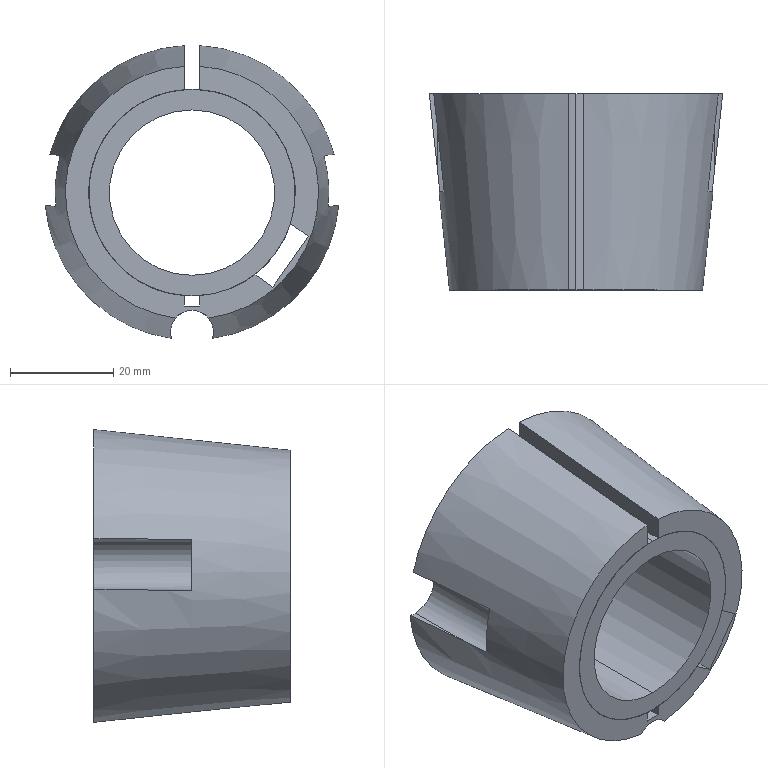Part | SolidWorks | features BaseBody 1, ICE 1 | 1 solid | 27 faces | box 56.795 x 38 x 56.678 mm | volume 48343 mm3 | plane 13 | cylinder 12 | cone 2 | commonest cylinder face diameters 10 x6 8.376 x2 32 x2 40 x2
STEP:
#1=CARTESIAN_POINT('',(0.,-0.0001031,-16.));
#2=VERTEX_POINT('',#1);
#3=CARTESIAN_POINT('',(0.,-0.0001031,16.));
#4=VERTEX_POINT('',#3);
#5=CARTESIAN_POINT('',(0.,-0.0001031,0.));
#6=DIRECTION('',(0.,1.,0.));
#7=DIRECTION('',(0.,0.,1.));
#8=AXIS2_PLACEMENT_3D('',#5,#6,#7);
#9=CIRCLE('',#8,16.);
#10=EDGE_CURVE('',#2,#4,#9,.T.);
#11=ORIENTED_EDGE('',*,*,#10,.F.);
#12=CARTESIAN_POINT('',(0.,38.,-16.));
#13=VERTEX_POINT('',#12);
#14=CARTESIAN_POINT('',(0.,-0.0001031,-16.));
#15=DIRECTION('',(0.,1.,0.));
#16=VECTOR('',#15,1000.);
#17=LINE('',#14,#16);
#18=EDGE_CURVE('',#2,#13,#17,.T.);
#19=ORIENTED_EDGE('',*,*,#18,.T.);
#20=CARTESIAN_POINT('',(0.,38.,16.));
#21=VERTEX_POINT('',#20);
#22=CARTESIAN_POINT('',(0.,38.,0.));
#23=DIRECTION('',(0.,1.,0.));
#24=DIRECTION('',(0.,0.,1.));
#25=AXIS2_PLACEMENT_3D('',#22,#23,#24);
#26=CIRCLE('',#25,16.);
#27=EDGE_CURVE('',#13,#21,#26,.T.);
#28=ORIENTED_EDGE('',*,*,#27,.T.);
#29=CARTESIAN_POINT('',(0.,-0.0001031,16.));
#30=DIRECTION('',(0.,1.,0.));
#31=VECTOR('',#30,1000.);
#32=LINE('',#29,#31);
#33=EDGE_CURVE('',#4,#21,#32,.T.);
#34=ORIENTED_EDGE('',*,*,#33,.F.);
#35=EDGE_LOOP('',(#11,#19,#28,#34));
#36=FACE_OUTER_BOUND('',#35,.T.);
#37=CARTESIAN_POINT('',(0.,-0.0001031,0.));
#38=DIRECTION('',(0.,1.,0.));
#39=DIRECTION('',(0.,0.,1.));
#40=AXIS2_PLACEMENT_3D('',#37,#38,#39);
#41=CYLINDRICAL_SURFACE('',#40,16.);
#42=ADVANCED_FACE('',(#36),#41,.F.);
#43=CARTESIAN_POINT('',(0.,-0.0001031,20.));
#44=VERTEX_POINT('',#43);
#45=CARTESIAN_POINT('',(0.,-0.0001031,-20.));
#46=VERTEX_POINT('',#45);
#47=CARTESIAN_POINT('',(0.,-0.0001031,0.));
#48=DIRECTION('',(0.,1.,0.));
#49=DIRECTION('',(0.,0.,1.));
#50=AXIS2_PLACEMENT_3D('',#47,#48,#49);
#51=CIRCLE('',#50,20.);
#52=EDGE_CURVE('',#44,#46,#51,.T.);
#53=ORIENTED_EDGE('',*,*,#52,.T.);
#54=CARTESIAN_POINT('',(0.,38.,-20.));
#55=VERTEX_POINT('',#54);
#56=CARTESIAN_POINT('',(0.,-0.0001031,-20.));
#57=DIRECTION('',(0.,1.,0.));
#58=VECTOR('',#57,1000.);
#59=LINE('',#56,#58);
#60=EDGE_CURVE('',#46,#55,#59,.T.);
#61=ORIENTED_EDGE('',*,*,#60,.T.);
#62=CARTESIAN_POINT('',(1.5,38.,-19.944));
#63=VERTEX_POINT('',#62);
#64=CARTESIAN_POINT('',(0.,38.,0.));
#65=DIRECTION('',(0.,1.,0.));
#66=DIRECTION('',(0.,0.,1.));
#67=AXIS2_PLACEMENT_3D('',#64,#65,#66);
#68=CIRCLE('',#67,20.);
#69=EDGE_CURVE('',#63,#55,#68,.T.);
#70=ORIENTED_EDGE('',*,*,#69,.F.);
#71=CARTESIAN_POINT('',(1.5,0.,-19.944));
#72=VERTEX_POINT('',#71);
#73=CARTESIAN_POINT('',(1.5,-50.,-19.944));
#74=DIRECTION('',(0.,1.,0.));
#75=VECTOR('',#74,1000.);
#76=LINE('',#73,#75);
#77=EDGE_CURVE('',#72,#63,#76,.T.);
#78=ORIENTED_EDGE('',*,*,#77,.F.);
#79=CARTESIAN_POINT('',(12.187,0.,-15.858));
#80=VERTEX_POINT('',#79);
#81=CARTESIAN_POINT('',(0.,0.,0.));
#82=DIRECTION('',(0.,1.,0.));
#83=DIRECTION('',(0.,0.,1.));
#84=AXIS2_PLACEMENT_3D('',#81,#82,#83);
#85=CIRCLE('',#84,20.);
#86=EDGE_CURVE('',#80,#72,#85,.T.);
#87=ORIENTED_EDGE('',*,*,#86,.F.);
#88=CARTESIAN_POINT('',(12.187,38.,-15.858));
#89=VERTEX_POINT('',#88);
#90=CARTESIAN_POINT('',(12.187,-462.,-15.858));
#91=DIRECTION('',(0.,1.,0.));
#92=VECTOR('',#91,1000.);
#93=LINE('',#90,#92);
#94=EDGE_CURVE('',#80,#89,#93,.T.);
#95=ORIENTED_EDGE('',*,*,#94,.T.);
#96=CARTESIAN_POINT('',(19.07,38.,-6.028));
#97=VERTEX_POINT('',#96);
#98=CARTESIAN_POINT('',(0.,38.,0.));
#99=DIRECTION('',(0.,1.,0.));
#100=DIRECTION('',(0.,0.,1.));
#101=AXIS2_PLACEMENT_3D('',#98,#99,#100);
#102=CIRCLE('',#101,20.);
#103=EDGE_CURVE('',#97,#89,#102,.T.);
#104=ORIENTED_EDGE('',*,*,#103,.F.);
#105=CARTESIAN_POINT('',(19.07,0.,-6.028));
#106=VERTEX_POINT('',#105);
#107=CARTESIAN_POINT('',(19.07,-50.,-6.028));
#108=DIRECTION('',(0.,1.,0.));
#109=VECTOR('',#108,1000.);
#110=LINE('',#107,#109);
#111=EDGE_CURVE('',#106,#97,#110,.T.);
#112=ORIENTED_EDGE('',*,*,#111,.F.);
#113=CARTESIAN_POINT('',(1.5,0.,19.944));
#114=VERTEX_POINT('',#113);
#115=CARTESIAN_POINT('',(0.,0.,0.));
#116=DIRECTION('',(0.,1.,0.));
#117=DIRECTION('',(0.,0.,1.));
#118=AXIS2_PLACEMENT_3D('',#115,#116,#117);
#119=CIRCLE('',#118,20.);
#120=EDGE_CURVE('',#114,#106,#119,.T.);
#121=ORIENTED_EDGE('',*,*,#120,.F.);
#122=CARTESIAN_POINT('',(1.5,38.,19.944));
#123=VERTEX_POINT('',#122);
#124=CARTESIAN_POINT('',(1.5,-462.,19.944));
#125=DIRECTION('',(0.,1.,0.));
#126=VECTOR('',#125,1000.);
#127=LINE('',#124,#126);
#128=EDGE_CURVE('',#114,#123,#127,.T.);
#129=ORIENTED_EDGE('',*,*,#128,.T.);
#130=CARTESIAN_POINT('',(0.,38.,20.));
#131=VERTEX_POINT('',#130);
#132=CARTESIAN_POINT('',(0.,38.,0.));
#133=DIRECTION('',(0.,1.,0.));
#134=DIRECTION('',(0.,0.,1.));
#135=AXIS2_PLACEMENT_3D('',#132,#133,#134);
#136=CIRCLE('',#135,20.);
#137=EDGE_CURVE('',#131,#123,#136,.T.);
#138=ORIENTED_EDGE('',*,*,#137,.F.);
#139=CARTESIAN_POINT('',(0.,-0.0001031,20.));
#140=DIRECTION('',(0.,1.,0.));
#141=VECTOR('',#140,1000.);
#142=LINE('',#139,#141);
#143=EDGE_CURVE('',#44,#131,#142,.T.);
#144=ORIENTED_EDGE('',*,*,#143,.F.);
#145=EDGE_LOOP('',(#53,#61,#70,#78,#87,#95,#104,#112,#121,#129,#138,#144));
#146=FACE_OUTER_BOUND('',#145,.T.);
#147=CARTESIAN_POINT('',(0.,-0.0001031,0.));
#148=DIRECTION('',(0.,1.,0.));
#149=DIRECTION('',(0.,0.,1.));
#150=AXIS2_PLACEMENT_3D('',#147,#148,#149);
#151=CYLINDRICAL_SURFACE('',#150,20.);
#152=ADVANCED_FACE('',(#146),#151,.T.);
#153=CARTESIAN_POINT('',(26.885,38.,7.352));
#154=VERTEX_POINT('',#153);
#155=CARTESIAN_POINT('',(26.885,38.,-2.648));
#156=VERTEX_POINT('',#155);
#157=CARTESIAN_POINT('',(26.885,38.,2.352));
#158=DIRECTION('',(0.,-1.,0.));
#159=DIRECTION('',(0.,0.,-1.));
#160=AXIS2_PLACEMENT_3D('',#157,#158,#159);
#161=CIRCLE('',#160,5.);
#162=EDGE_CURVE('',#154,#156,#161,.T.);
#163=ORIENTED_EDGE('',*,*,#162,.F.);
#164=CARTESIAN_POINT('',(26.885,32.025,7.352));
#165=VERTEX_POINT('',#164);
#166=CARTESIAN_POINT('',(26.885,19.,7.352));
#167=DIRECTION('',(0.,-1.,0.));
#168=VECTOR('',#167,1000.);
#169=LINE('',#166,#168);
#170=EDGE_CURVE('',#154,#165,#169,.T.);
#171=ORIENTED_EDGE('',*,*,#170,.T.);
#172=CARTESIAN_POINT('',(25.517,19.,7.161));
#173=VERTEX_POINT('',#172);
#174=CARTESIAN_POINT('',(25.517,19.,7.161));
#175=CARTESIAN_POINT('',(25.956,23.342,7.286));
#176=CARTESIAN_POINT('',(26.412,27.684,7.352));
#177=CARTESIAN_POINT('',(26.885,32.025,7.352));
#178=B_SPLINE_CURVE_WITH_KNOTS('',3,(#174,#175,#176,#177),.UNSPECIFIED.,.F.,.F.,(4,4),(0.,0.0131),.UNSPECIFIED.);
#179=EDGE_CURVE('',#173,#165,#178,.T.);
#180=ORIENTED_EDGE('',*,*,#179,.F.);
#181=CARTESIAN_POINT('',(26.373,19.,-2.622));
#182=VERTEX_POINT('',#181);
#183=CARTESIAN_POINT('',(26.885,19.,2.352));
#184=DIRECTION('',(0.,1.,0.));
#185=DIRECTION('',(0.,0.,-1.));
#186=AXIS2_PLACEMENT_3D('',#183,#184,#185);
#187=CIRCLE('',#186,5.);
#188=EDGE_CURVE('',#182,#173,#187,.T.);
#189=ORIENTED_EDGE('',*,*,#188,.F.);
#190=CARTESIAN_POINT('',(26.885,23.87,-2.648));
#191=VERTEX_POINT('',#190);
#192=CARTESIAN_POINT('',(26.885,23.87,-2.648));
#193=CARTESIAN_POINT('',(26.713,22.247,-2.648));
#194=CARTESIAN_POINT('',(26.543,20.623,-2.639));
#195=CARTESIAN_POINT('',(26.373,19.,-2.622));
#196=B_SPLINE_CURVE_WITH_KNOTS('',3,(#192,#193,#194,#195),.UNSPECIFIED.,.F.,.F.,(4,4),(0.01421,0.01911),.UNSPECIFIED.);
#197=EDGE_CURVE('',#191,#182,#196,.T.);
#198=ORIENTED_EDGE('',*,*,#197,.F.);
#199=CARTESIAN_POINT('',(26.885,19.,-2.648));
#200=DIRECTION('',(0.,-1.,0.));
#201=VECTOR('',#200,1000.);
#202=LINE('',#199,#201);
#203=EDGE_CURVE('',#156,#191,#202,.T.);
#204=ORIENTED_EDGE('',*,*,#203,.F.);
#205=EDGE_LOOP('',(#163,#171,#180,#189,#198,#204));
#206=FACE_OUTER_BOUND('',#205,.T.);
#207=CARTESIAN_POINT('',(26.885,19.,2.352));
#208=DIRECTION('',(0.,-1.,0.));
#209=DIRECTION('',(0.,0.,-1.));
#210=AXIS2_PLACEMENT_3D('',#207,#208,#209);
#211=CYLINDRICAL_SURFACE('',#210,5.);
#212=ADVANCED_FACE('',(#206),#211,.F.);
#213=CARTESIAN_POINT('',(28.398,38.,-2.414));
#214=VERTEX_POINT('',#213);
#215=CARTESIAN_POINT('',(26.885,38.,2.352));
#216=DIRECTION('',(0.,-1.,0.));
#217=DIRECTION('',(0.,0.,-1.));
#218=AXIS2_PLACEMENT_3D('',#215,#216,#217);
#219=CIRCLE('',#218,5.);
#220=EDGE_CURVE('',#156,#214,#219,.T.);
#221=ORIENTED_EDGE('',*,*,#220,.F.);
#222=ORIENTED_EDGE('',*,*,#203,.T.);
#223=CARTESIAN_POINT('',(28.398,38.,-2.414));
#224=CARTESIAN_POINT('',(27.887,33.292,-2.576));
#225=CARTESIAN_POINT('',(27.382,28.582,-2.648));
#226=CARTESIAN_POINT('',(26.885,23.87,-2.648));
#227=B_SPLINE_CURVE_WITH_KNOTS('',3,(#223,#224,#225,#226),.UNSPECIFIED.,.F.,.F.,(4,4),(0.,0.01421),.UNSPECIFIED.);
#228=EDGE_CURVE('',#214,#191,#227,.T.);
#229=ORIENTED_EDGE('',*,*,#228,.F.);
#230=EDGE_LOOP('',(#221,#222,#229));
#231=FACE_OUTER_BOUND('',#230,.T.);
#232=CARTESIAN_POINT('',(26.885,19.,2.352));
#233=DIRECTION('',(0.,-1.,0.));
#234=DIRECTION('',(0.,0.,-1.));
#235=AXIS2_PLACEMENT_3D('',#232,#233,#234);
#236=CYLINDRICAL_SURFACE('',#235,5.);
#237=ADVANCED_FACE('',(#231),#236,.F.);
#238=CARTESIAN_POINT('',(0.,0.,-22.8));
#239=VERTEX_POINT('',#238);
#240=CARTESIAN_POINT('',(3.208,0.,-24.295));
#241=VERTEX_POINT('',#240);
#242=CARTESIAN_POINT('',(0.,0.,-26.988));
#243=DIRECTION('',(0.,1.,0.));
#244=DIRECTION('',(0.,0.,1.));
#245=AXIS2_PLACEMENT_3D('',#242,#243,#244);
#246=CIRCLE('',#245,4.188);
#247=EDGE_CURVE('',#239,#241,#246,.T.);
#248=ORIENTED_EDGE('',*,*,#247,.F.);
#249=CARTESIAN_POINT('',(0.,38.,-22.8));
#250=VERTEX_POINT('',#249);
#251=CARTESIAN_POINT('',(0.,0.,-22.8));
#252=DIRECTION('',(0.,1.,0.));
#253=VECTOR('',#252,1000.);
#254=LINE('',#251,#253);
#255=EDGE_CURVE('',#239,#250,#254,.T.);
#256=ORIENTED_EDGE('',*,*,#255,.T.);
#257=CARTESIAN_POINT('',(4.003,38.,-28.217));
#258=VERTEX_POINT('',#257);
#259=CARTESIAN_POINT('',(0.,38.,-26.988));
#260=DIRECTION('',(0.,-1.,0.));
#261=DIRECTION('',(0.,0.,1.));
#262=AXIS2_PLACEMENT_3D('',#259,#260,#261);
#263=CIRCLE('',#262,4.188);
#264=EDGE_CURVE('',#258,#250,#263,.T.);
#265=ORIENTED_EDGE('',*,*,#264,.F.);
#266=CARTESIAN_POINT('',(3.208,0.,-24.295));
#267=CARTESIAN_POINT('',(3.461,3.163,-24.597));
#268=CARTESIAN_POINT('',(3.65,6.33,-24.905));
#269=CARTESIAN_POINT('',(3.943,12.665,-25.535));
#270=CARTESIAN_POINT('',(4.046,15.833,-25.855));
#271=CARTESIAN_POINT('',(4.174,22.167,-26.509));
#272=CARTESIAN_POINT('',(4.199,25.334,-26.842));
#273=CARTESIAN_POINT('',(4.168,31.667,-27.521));
#274=CARTESIAN_POINT('',(4.111,34.834,-27.866));
#275=CARTESIAN_POINT('',(4.003,38.,-28.217));
#276=B_SPLINE_CURVE_WITH_KNOTS('',3,(#266,#267,#268,#269,#270,#271,#272,#273,#274,#275),.UNSPECIFIED.,.F.,.F.,(4,2,2,2,4),(0.,0.009561,0.01912,0.02868,0.03824),.UNSPECIFIED.);
#277=EDGE_CURVE('',#241,#258,#276,.T.);
#278=ORIENTED_EDGE('',*,*,#277,.F.);
#279=EDGE_LOOP('',(#248,#256,#265,#278));
#280=FACE_OUTER_BOUND('',#279,.T.);
#281=CARTESIAN_POINT('',(0.,0.,-26.988));
#282=DIRECTION('',(0.,1.,0.));
#283=DIRECTION('',(0.,0.,1.));
#284=AXIS2_PLACEMENT_3D('',#281,#282,#283);
#285=CYLINDRICAL_SURFACE('',#284,4.188);
#286=ADVANCED_FACE('',(#280),#285,.F.);
#287=CARTESIAN_POINT('',(-26.885,38.,7.352));
#288=VERTEX_POINT('',#287);
#289=CARTESIAN_POINT('',(-27.547,38.,7.308));
#290=VERTEX_POINT('',#289);
#291=CARTESIAN_POINT('',(-26.885,38.,2.352));
#292=DIRECTION('',(0.,-1.,0.));
#293=DIRECTION('',(0.,0.,-1.));
#294=AXIS2_PLACEMENT_3D('',#291,#292,#293);
#295=CIRCLE('',#294,5.);
#296=EDGE_CURVE('',#288,#290,#295,.T.);
#297=ORIENTED_EDGE('',*,*,#296,.F.);
#298=CARTESIAN_POINT('',(-26.885,32.025,7.352));
#299=VERTEX_POINT('',#298);
#300=CARTESIAN_POINT('',(-26.885,19.,7.352));
#301=DIRECTION('',(0.,-1.,0.));
#302=VECTOR('',#301,1000.);
#303=LINE('',#300,#302);
#304=EDGE_CURVE('',#288,#299,#303,.T.);
#305=ORIENTED_EDGE('',*,*,#304,.T.);
#306=CARTESIAN_POINT('',(-27.547,38.,7.308));
#307=CARTESIAN_POINT('',(-27.323,36.009,7.338));
#308=CARTESIAN_POINT('',(-27.102,34.017,7.352));
#309=CARTESIAN_POINT('',(-26.885,32.025,7.352));
#310=B_SPLINE_CURVE_WITH_KNOTS('',3,(#306,#307,#308,#309),.UNSPECIFIED.,.F.,.F.,(4,4),(0.,0.006012),.UNSPECIFIED.);
#311=EDGE_CURVE('',#290,#299,#310,.T.);
#312=ORIENTED_EDGE('',*,*,#311,.F.);
#313=EDGE_LOOP('',(#297,#305,#312));
#314=FACE_OUTER_BOUND('',#313,.T.);
#315=CARTESIAN_POINT('',(-26.885,19.,2.352));
#316=DIRECTION('',(0.,-1.,0.));
#317=DIRECTION('',(0.,0.,-1.));
#318=AXIS2_PLACEMENT_3D('',#315,#316,#317);
#319=CYLINDRICAL_SURFACE('',#318,5.);
#320=ADVANCED_FACE('',(#314),#319,.F.);
#321=ORIENTED_EDGE('',*,*,#304,.F.);
#322=CARTESIAN_POINT('',(-26.885,38.,-2.648));
#323=VERTEX_POINT('',#322);
#324=CARTESIAN_POINT('',(-26.885,38.,2.352));
#325=DIRECTION('',(0.,-1.,0.));
#326=DIRECTION('',(0.,0.,-1.));
#327=AXIS2_PLACEMENT_3D('',#324,#325,#326);
#328=CIRCLE('',#327,5.);
#329=EDGE_CURVE('',#323,#288,#328,.T.);
#330=ORIENTED_EDGE('',*,*,#329,.F.);
#331=CARTESIAN_POINT('',(-26.885,23.87,-2.648));
#332=VERTEX_POINT('',#331);
#333=CARTESIAN_POINT('',(-26.885,19.,-2.648));
#334=DIRECTION('',(0.,-1.,0.));
#335=VECTOR('',#334,1000.);
#336=LINE('',#333,#335);
#337=EDGE_CURVE('',#323,#332,#336,.T.);
#338=ORIENTED_EDGE('',*,*,#337,.T.);
#339=CARTESIAN_POINT('',(-26.373,19.,-2.622));
#340=VERTEX_POINT('',#339);
#341=CARTESIAN_POINT('',(-26.373,19.,-2.622));
#342=CARTESIAN_POINT('',(-26.543,20.623,-2.639));
#343=CARTESIAN_POINT('',(-26.713,22.247,-2.648));
#344=CARTESIAN_POINT('',(-26.885,23.87,-2.648));
#345=B_SPLINE_CURVE_WITH_KNOTS('',3,(#341,#342,#343,#344),.UNSPECIFIED.,.F.,.F.,(4,4),(0.,0.004897),.UNSPECIFIED.);
#346=EDGE_CURVE('',#340,#332,#345,.T.);
#347=ORIENTED_EDGE('',*,*,#346,.F.);
#348=CARTESIAN_POINT('',(-25.517,19.,7.161));
#349=VERTEX_POINT('',#348);
#350=CARTESIAN_POINT('',(-26.885,19.,2.352));
#351=DIRECTION('',(0.,1.,0.));
#352=DIRECTION('',(0.,0.,-1.));
#353=AXIS2_PLACEMENT_3D('',#350,#351,#352);
#354=CIRCLE('',#353,5.);
#355=EDGE_CURVE('',#349,#340,#354,.T.);
#356=ORIENTED_EDGE('',*,*,#355,.F.);
#357=CARTESIAN_POINT('',(-26.885,32.025,7.352));
#358=CARTESIAN_POINT('',(-26.412,27.684,7.352));
#359=CARTESIAN_POINT('',(-25.956,23.342,7.286));
#360=CARTESIAN_POINT('',(-25.517,19.,7.161));
#361=B_SPLINE_CURVE_WITH_KNOTS('',3,(#357,#358,#359,#360),.UNSPECIFIED.,.F.,.F.,(4,4),(0.006012,0.01911),.UNSPECIFIED.);
#362=EDGE_CURVE('',#299,#349,#361,.T.);
#363=ORIENTED_EDGE('',*,*,#362,.F.);
#364=EDGE_LOOP('',(#321,#330,#338,#347,#356,#363));
#365=FACE_OUTER_BOUND('',#364,.T.);
#366=CARTESIAN_POINT('',(-26.885,19.,2.352));
#367=DIRECTION('',(0.,-1.,0.));
#368=DIRECTION('',(0.,0.,-1.));
#369=AXIS2_PLACEMENT_3D('',#366,#367,#368);
#370=CYLINDRICAL_SURFACE('',#369,5.);
#371=ADVANCED_FACE('',(#365),#370,.F.);
#372=ORIENTED_EDGE('',*,*,#228,.T.);
#373=ORIENTED_EDGE('',*,*,#197,.T.);
#374=CARTESIAN_POINT('',(0.,19.,0.));
#375=DIRECTION('',(0.,-1.,0.));
#376=DIRECTION('',(0.,0.,1.));
#377=AXIS2_PLACEMENT_3D('',#374,#375,#376);
#378=CIRCLE('',#377,26.503);
#379=EDGE_CURVE('',#182,#173,#378,.T.);
#380=ORIENTED_EDGE('',*,*,#379,.T.);
#381=ORIENTED_EDGE('',*,*,#179,.T.);
#382=CARTESIAN_POINT('',(27.547,38.,7.308));
#383=VERTEX_POINT('',#382);
#384=CARTESIAN_POINT('',(26.885,32.025,7.352));
#385=CARTESIAN_POINT('',(27.102,34.017,7.352));
#386=CARTESIAN_POINT('',(27.323,36.009,7.338));
#387=CARTESIAN_POINT('',(27.547,38.,7.308));
#388=B_SPLINE_CURVE_WITH_KNOTS('',3,(#384,#385,#386,#387),.UNSPECIFIED.,.F.,.F.,(4,4),(0.0131,0.01911),.UNSPECIFIED.);
#389=EDGE_CURVE('',#165,#383,#388,.T.);
#390=ORIENTED_EDGE('',*,*,#389,.T.);
#391=CARTESIAN_POINT('',(1.5,38.,28.46));
#392=VERTEX_POINT('',#391);
#393=CARTESIAN_POINT('',(0.,38.,0.));
#394=DIRECTION('',(0.,-1.,0.));
#395=DIRECTION('',(0.,0.,1.));
#396=AXIS2_PLACEMENT_3D('',#393,#394,#395);
#397=CIRCLE('',#396,28.5);
#398=EDGE_CURVE('',#383,#392,#397,.T.);
#399=ORIENTED_EDGE('',*,*,#398,.T.);
#400=CARTESIAN_POINT('',(1.5,0.,24.46));
#401=VERTEX_POINT('',#400);
#402=CARTESIAN_POINT('',(1.5,38.,28.46));
#403=CARTESIAN_POINT('',(1.5,25.333,27.127));
#404=CARTESIAN_POINT('',(1.5,12.667,25.794));
#405=CARTESIAN_POINT('',(1.5,0.,24.46));
#406=B_SPLINE_CURVE_WITH_KNOTS('',3,(#402,#403,#404,#405),.UNSPECIFIED.,.F.,.F.,(4,4),(0.,0.03821),.UNSPECIFIED.);
#407=EDGE_CURVE('',#392,#401,#406,.T.);
#408=ORIENTED_EDGE('',*,*,#407,.T.);
#409=CARTESIAN_POINT('',(0.,0.,0.));
#410=DIRECTION('',(0.,1.,0.));
#411=DIRECTION('',(0.,0.,1.));
#412=AXIS2_PLACEMENT_3D('',#409,#410,#411);
#413=CIRCLE('',#412,24.506);
#414=EDGE_CURVE('',#401,#241,#413,.T.);
#415=ORIENTED_EDGE('',*,*,#414,.T.);
#416=ORIENTED_EDGE('',*,*,#277,.T.);
#417=CARTESIAN_POINT('',(0.,38.,0.));
#418=DIRECTION('',(0.,-1.,0.));
#419=DIRECTION('',(0.,0.,1.));
#420=AXIS2_PLACEMENT_3D('',#417,#418,#419);
#421=CIRCLE('',#420,28.5);
#422=EDGE_CURVE('',#258,#214,#421,.T.);
#423=ORIENTED_EDGE('',*,*,#422,.T.);
#424=EDGE_LOOP('',(#372,#373,#380,#381,#390,#399,#408,#415,#416,#423));
#425=FACE_OUTER_BOUND('',#424,.T.);
#426=CARTESIAN_POINT('',(0.,38.,0.));
#427=DIRECTION('',(0.,1.,0.));
#428=DIRECTION('',(0.,0.,1.));
#429=AXIS2_PLACEMENT_3D('',#426,#427,#428);
#430=CONICAL_SURFACE('',#429,28.5,0.1047);
#431=ADVANCED_FACE('',(#425),#430,.T.);
#432=ORIENTED_EDGE('',*,*,#188,.T.);
#433=ORIENTED_EDGE('',*,*,#379,.F.);
#434=EDGE_LOOP('',(#432,#433));
#435=FACE_OUTER_BOUND('',#434,.T.);
#436=CARTESIAN_POINT('',(0.,19.,0.));
#437=DIRECTION('',(0.,1.,0.));
#438=DIRECTION('',(0.,0.,1.));
#439=AXIS2_PLACEMENT_3D('',#436,#437,#438);
#440=PLANE('',#439);
#441=ADVANCED_FACE('',(#435),#440,.T.);
#442=ORIENTED_EDGE('',*,*,#170,.F.);
#443=CARTESIAN_POINT('',(26.885,38.,2.352));
#444=DIRECTION('',(0.,-1.,0.));
#445=DIRECTION('',(0.,0.,-1.));
#446=AXIS2_PLACEMENT_3D('',#443,#444,#445);
#447=CIRCLE('',#446,5.);
#448=EDGE_CURVE('',#383,#154,#447,.T.);
#449=ORIENTED_EDGE('',*,*,#448,.F.);
#450=ORIENTED_EDGE('',*,*,#389,.F.);
#451=EDGE_LOOP('',(#442,#449,#450));
#452=FACE_OUTER_BOUND('',#451,.T.);
#453=CARTESIAN_POINT('',(26.885,19.,2.352));
#454=DIRECTION('',(0.,-1.,0.));
#455=DIRECTION('',(0.,0.,-1.));
#456=AXIS2_PLACEMENT_3D('',#453,#454,#455);
#457=CYLINDRICAL_SURFACE('',#456,5.);
#458=ADVANCED_FACE('',(#452),#457,.F.);
#459=CARTESIAN_POINT('',(-1.5,38.,19.944));
#460=VERTEX_POINT('',#459);
#461=CARTESIAN_POINT('',(0.,38.,0.));
#462=DIRECTION('',(0.,1.,0.));
#463=DIRECTION('',(0.,0.,1.));
#464=AXIS2_PLACEMENT_3D('',#461,#462,#463);
#465=CIRCLE('',#464,20.);
#466=EDGE_CURVE('',#460,#131,#465,.T.);
#467=ORIENTED_EDGE('',*,*,#466,.T.);
#468=ORIENTED_EDGE('',*,*,#137,.T.);
#469=CARTESIAN_POINT('',(1.5,38.,0.));
#470=DIRECTION('',(0.,0.,1.));
#471=VECTOR('',#470,1000.);
#472=LINE('',#469,#471);
#473=EDGE_CURVE('',#123,#392,#472,.T.);
#474=ORIENTED_EDGE('',*,*,#473,.T.);
#475=ORIENTED_EDGE('',*,*,#398,.F.);
#476=ORIENTED_EDGE('',*,*,#448,.T.);
#477=ORIENTED_EDGE('',*,*,#162,.T.);
#478=ORIENTED_EDGE('',*,*,#220,.T.);
#479=ORIENTED_EDGE('',*,*,#422,.F.);
#480=ORIENTED_EDGE('',*,*,#264,.T.);
#481=CARTESIAN_POINT('',(-4.003,38.,-28.217));
#482=VERTEX_POINT('',#481);
#483=CARTESIAN_POINT('',(0.,38.,-26.988));
#484=DIRECTION('',(0.,-1.,0.));
#485=DIRECTION('',(0.,0.,1.));
#486=AXIS2_PLACEMENT_3D('',#483,#484,#485);
#487=CIRCLE('',#486,4.188);
#488=EDGE_CURVE('',#250,#482,#487,.T.);
#489=ORIENTED_EDGE('',*,*,#488,.T.);
#490=CARTESIAN_POINT('',(-28.398,38.,-2.414));
#491=VERTEX_POINT('',#490);
#492=CARTESIAN_POINT('',(0.,38.,0.));
#493=DIRECTION('',(0.,1.,0.));
#494=DIRECTION('',(0.,0.,1.));
#495=AXIS2_PLACEMENT_3D('',#492,#493,#494);
#496=CIRCLE('',#495,28.5);
#497=EDGE_CURVE('',#482,#491,#496,.T.);
#498=ORIENTED_EDGE('',*,*,#497,.T.);
#499=CARTESIAN_POINT('',(-26.885,38.,2.352));
#500=DIRECTION('',(0.,-1.,0.));
#501=DIRECTION('',(0.,0.,-1.));
#502=AXIS2_PLACEMENT_3D('',#499,#500,#501);
#503=CIRCLE('',#502,5.);
#504=EDGE_CURVE('',#491,#323,#503,.T.);
#505=ORIENTED_EDGE('',*,*,#504,.T.);
#506=ORIENTED_EDGE('',*,*,#329,.T.);
#507=ORIENTED_EDGE('',*,*,#296,.T.);
#508=CARTESIAN_POINT('',(-1.5,38.,28.46));
#509=VERTEX_POINT('',#508);
#510=CARTESIAN_POINT('',(0.,38.,0.));
#511=DIRECTION('',(0.,1.,0.));
#512=DIRECTION('',(0.,0.,1.));
#513=AXIS2_PLACEMENT_3D('',#510,#511,#512);
#514=CIRCLE('',#513,28.5);
#515=EDGE_CURVE('',#290,#509,#514,.T.);
#516=ORIENTED_EDGE('',*,*,#515,.T.);
#517=CARTESIAN_POINT('',(-1.5,38.,0.));
#518=DIRECTION('',(0.,0.,-1.));
#519=VECTOR('',#518,1000.);
#520=LINE('',#517,#519);
#521=EDGE_CURVE('',#509,#460,#520,.T.);
#522=ORIENTED_EDGE('',*,*,#521,.T.);
#523=EDGE_LOOP('',(#467,#468,#474,#475,#476,#477,#478,#479,#480,#489,#498,#505,#506,#507,#516,#522));
#524=FACE_OUTER_BOUND('',#523,.T.);
#525=ORIENTED_EDGE('',*,*,#103,.T.);
#526=CARTESIAN_POINT('',(15.645,38.,-18.279));
#527=VERTEX_POINT('',#526);
#528=CARTESIAN_POINT('',(12.187,38.,-15.858));
#529=DIRECTION('',(0.8192,0.,-0.5736));
#530=VECTOR('',#529,1000.);
#531=LINE('',#528,#530);
#532=EDGE_CURVE('',#89,#527,#531,.T.);
#533=ORIENTED_EDGE('',*,*,#532,.T.);
#534=CARTESIAN_POINT('',(22.528,38.,-8.449));
#535=VERTEX_POINT('',#534);
#536=CARTESIAN_POINT('',(15.645,38.,-18.279));
#537=DIRECTION('',(0.5736,0.,0.8192));
#538=VECTOR('',#537,1000.);
#539=LINE('',#536,#538);
#540=EDGE_CURVE('',#527,#535,#539,.T.);
#541=ORIENTED_EDGE('',*,*,#540,.T.);
#542=CARTESIAN_POINT('',(22.528,38.,-8.449));
#543=DIRECTION('',(-0.8192,0.,0.5736));
#544=VECTOR('',#543,1000.);
#545=LINE('',#542,#544);
#546=EDGE_CURVE('',#535,#97,#545,.T.);
#547=ORIENTED_EDGE('',*,*,#546,.T.);
#548=EDGE_LOOP('',(#525,#533,#541,#547));
#549=FACE_BOUND('',#548,.T.);
#550=CARTESIAN_POINT('',(1.5,38.,-21.949));
#551=VERTEX_POINT('',#550);
#552=CARTESIAN_POINT('',(1.5,38.,0.));
#553=DIRECTION('',(0.,0.,1.));
#554=VECTOR('',#553,1000.);
#555=LINE('',#552,#554);
#556=EDGE_CURVE('',#551,#63,#555,.T.);
#557=ORIENTED_EDGE('',*,*,#556,.T.);
#558=ORIENTED_EDGE('',*,*,#69,.T.);
#559=CARTESIAN_POINT('',(-1.5,38.,-19.944));
#560=VERTEX_POINT('',#559);
#561=CARTESIAN_POINT('',(0.,38.,0.));
#562=DIRECTION('',(0.,1.,0.));
#563=DIRECTION('',(0.,0.,1.));
#564=AXIS2_PLACEMENT_3D('',#561,#562,#563);
#565=CIRCLE('',#564,20.);
#566=EDGE_CURVE('',#55,#560,#565,.T.);
#567=ORIENTED_EDGE('',*,*,#566,.T.);
#568=CARTESIAN_POINT('',(-1.5,38.,-21.949));
#569=VERTEX_POINT('',#568);
#570=CARTESIAN_POINT('',(-1.5,38.,0.));
#571=DIRECTION('',(0.,0.,-1.));
#572=VECTOR('',#571,1000.);
#573=LINE('',#570,#572);
#574=EDGE_CURVE('',#560,#569,#573,.T.);
#575=ORIENTED_EDGE('',*,*,#574,.T.);
#576=CARTESIAN_POINT('',(28.5,38.,-21.949));
#577=DIRECTION('',(1.,0.,0.));
#578=VECTOR('',#577,1000.);
#579=LINE('',#576,#578);
#580=EDGE_CURVE('',#569,#551,#579,.T.);
#581=ORIENTED_EDGE('',*,*,#580,.T.);
#582=EDGE_LOOP('',(#557,#558,#567,#575,#581));
#583=FACE_BOUND('',#582,.T.);
#584=CARTESIAN_POINT('',(0.,38.,0.));
#585=DIRECTION('',(0.,1.,0.));
#586=DIRECTION('',(0.,0.,1.));
#587=AXIS2_PLACEMENT_3D('',#584,#585,#586);
#588=CIRCLE('',#587,16.);
#589=EDGE_CURVE('',#21,#13,#588,.T.);
#590=ORIENTED_EDGE('',*,*,#589,.F.);
#591=ORIENTED_EDGE('',*,*,#27,.F.);
#592=EDGE_LOOP('',(#590,#591));
#593=FACE_BOUND('',#592,.T.);
#594=CARTESIAN_POINT('',(28.5,38.,0.));
#595=DIRECTION('',(0.,1.,0.));
#596=DIRECTION('',(0.,0.,1.));
#597=AXIS2_PLACEMENT_3D('',#594,#595,#596);
#598=PLANE('',#597);
#599=ADVANCED_FACE('',(#524,#549,#583,#593),#598,.T.);
#600=ORIENTED_EDGE('',*,*,#255,.F.);
#601=CARTESIAN_POINT('',(-3.208,0.,-24.295));
#602=VERTEX_POINT('',#601);
#603=CARTESIAN_POINT('',(0.,0.,-26.988));
#604=DIRECTION('',(0.,1.,0.));
#605=DIRECTION('',(0.,0.,1.));
#606=AXIS2_PLACEMENT_3D('',#603,#604,#605);
#607=CIRCLE('',#606,4.188);
#608=EDGE_CURVE('',#602,#239,#607,.T.);
#609=ORIENTED_EDGE('',*,*,#608,.F.);
#610=CARTESIAN_POINT('',(-4.003,38.,-28.217));
#611=CARTESIAN_POINT('',(-4.111,34.834,-27.866));
#612=CARTESIAN_POINT('',(-4.168,31.666,-27.521));
#613=CARTESIAN_POINT('',(-4.199,25.329,-26.842));
#614=CARTESIAN_POINT('',(-4.174,22.161,-26.509));
#615=CARTESIAN_POINT('',(-4.046,15.827,-25.855));
#616=CARTESIAN_POINT('',(-3.943,12.66,-25.534));
#617=CARTESIAN_POINT('',(-3.65,6.329,-24.905));
#618=CARTESIAN_POINT('',(-3.461,3.164,-24.597));
#619=CARTESIAN_POINT('',(-3.208,0.,-24.295));
#620=B_SPLINE_CURVE_WITH_KNOTS('',3,(#610,#611,#612,#613,#614,#615,#616,#617,#618,#619),.UNSPECIFIED.,.F.,.F.,(4,2,2,2,4),(0.,0.009561,0.01912,0.02868,0.03824),.UNSPECIFIED.);
#621=EDGE_CURVE('',#482,#602,#620,.T.);
#622=ORIENTED_EDGE('',*,*,#621,.F.);
#623=ORIENTED_EDGE('',*,*,#488,.F.);
#624=EDGE_LOOP('',(#600,#609,#622,#623));
#625=FACE_OUTER_BOUND('',#624,.T.);
#626=CARTESIAN_POINT('',(0.,0.,-26.988));
#627=DIRECTION('',(0.,1.,0.));
#628=DIRECTION('',(0.,0.,1.));
#629=AXIS2_PLACEMENT_3D('',#626,#627,#628);
#630=CYLINDRICAL_SURFACE('',#629,4.188);
#631=ADVANCED_FACE('',(#625),#630,.F.);
#632=ORIENTED_EDGE('',*,*,#608,.T.);
#633=ORIENTED_EDGE('',*,*,#247,.T.);
#634=ORIENTED_EDGE('',*,*,#414,.F.);
#635=CARTESIAN_POINT('',(1.5,0.,0.));
#636=DIRECTION('',(0.,0.,-1.));
#637=VECTOR('',#636,1000.);
#638=LINE('',#635,#637);
#639=EDGE_CURVE('',#401,#114,#638,.T.);
#640=ORIENTED_EDGE('',*,*,#639,.T.);
#641=ORIENTED_EDGE('',*,*,#120,.T.);
#642=CARTESIAN_POINT('',(22.528,0.,-8.449));
#643=VERTEX_POINT('',#642);
#644=CARTESIAN_POINT('',(19.07,0.,-6.028));
#645=DIRECTION('',(0.8192,0.,-0.5736));
#646=VECTOR('',#645,1000.);
#647=LINE('',#644,#646);
#648=EDGE_CURVE('',#106,#643,#647,.T.);
#649=ORIENTED_EDGE('',*,*,#648,.T.);
#650=CARTESIAN_POINT('',(15.645,0.,-18.279));
#651=VERTEX_POINT('',#650);
#652=CARTESIAN_POINT('',(22.528,0.,-8.449));
#653=DIRECTION('',(-0.5736,0.,-0.8192));
#654=VECTOR('',#653,1000.);
#655=LINE('',#652,#654);
#656=EDGE_CURVE('',#643,#651,#655,.T.);
#657=ORIENTED_EDGE('',*,*,#656,.T.);
#658=CARTESIAN_POINT('',(15.645,0.,-18.279));
#659=DIRECTION('',(-0.8192,0.,0.5736));
#660=VECTOR('',#659,1000.);
#661=LINE('',#658,#660);
#662=EDGE_CURVE('',#651,#80,#661,.T.);
#663=ORIENTED_EDGE('',*,*,#662,.T.);
#664=ORIENTED_EDGE('',*,*,#86,.T.);
#665=CARTESIAN_POINT('',(1.5,0.,-21.949));
#666=VERTEX_POINT('',#665);
#667=CARTESIAN_POINT('',(1.5,0.,0.));
#668=DIRECTION('',(0.,0.,-1.));
#669=VECTOR('',#668,1000.);
#670=LINE('',#667,#669);
#671=EDGE_CURVE('',#72,#666,#670,.T.);
#672=ORIENTED_EDGE('',*,*,#671,.T.);
#673=CARTESIAN_POINT('',(-1.5,0.,-21.949));
#674=VERTEX_POINT('',#673);
#675=CARTESIAN_POINT('',(20.,0.,-21.949));
#676=DIRECTION('',(-1.,0.,0.));
#677=VECTOR('',#676,1000.);
#678=LINE('',#675,#677);
#679=EDGE_CURVE('',#666,#674,#678,.T.);
#680=ORIENTED_EDGE('',*,*,#679,.T.);
#681=CARTESIAN_POINT('',(-1.5,0.,-19.944));
#682=VERTEX_POINT('',#681);
#683=CARTESIAN_POINT('',(-1.5,0.,0.));
#684=DIRECTION('',(0.,0.,1.));
#685=VECTOR('',#684,1000.);
#686=LINE('',#683,#685);
#687=EDGE_CURVE('',#674,#682,#686,.T.);
#688=ORIENTED_EDGE('',*,*,#687,.T.);
#689=CARTESIAN_POINT('',(-1.5,0.,19.944));
#690=VERTEX_POINT('',#689);
#691=CARTESIAN_POINT('',(0.,0.,0.));
#692=DIRECTION('',(0.,1.,0.));
#693=DIRECTION('',(0.,0.,1.));
#694=AXIS2_PLACEMENT_3D('',#691,#692,#693);
#695=CIRCLE('',#694,20.);
#696=EDGE_CURVE('',#682,#690,#695,.T.);
#697=ORIENTED_EDGE('',*,*,#696,.T.);
#698=CARTESIAN_POINT('',(-1.5,0.,24.46));
#699=VERTEX_POINT('',#698);
#700=CARTESIAN_POINT('',(-1.5,0.,0.));
#701=DIRECTION('',(0.,0.,1.));
#702=VECTOR('',#701,1000.);
#703=LINE('',#700,#702);
#704=EDGE_CURVE('',#690,#699,#703,.T.);
#705=ORIENTED_EDGE('',*,*,#704,.T.);
#706=CARTESIAN_POINT('',(0.,0.,0.));
#707=DIRECTION('',(0.,-1.,0.));
#708=DIRECTION('',(0.,0.,1.));
#709=AXIS2_PLACEMENT_3D('',#706,#707,#708);
#710=CIRCLE('',#709,24.506);
#711=EDGE_CURVE('',#699,#602,#710,.T.);
#712=ORIENTED_EDGE('',*,*,#711,.T.);
#713=EDGE_LOOP('',(#632,#633,#634,#640,#641,#649,#657,#663,#664,#672,#680,#688,#697,#705,#712));
#714=FACE_OUTER_BOUND('',#713,.T.);
#715=CARTESIAN_POINT('',(20.,0.,0.));
#716=DIRECTION('',(0.,-1.,0.));
#717=DIRECTION('',(0.,0.,-1.));
#718=AXIS2_PLACEMENT_3D('',#715,#716,#717);
#719=PLANE('',#718);
#720=ADVANCED_FACE('',(#714),#719,.T.);
#721=ORIENTED_EDGE('',*,*,#407,.F.);
#722=ORIENTED_EDGE('',*,*,#473,.F.);
#723=ORIENTED_EDGE('',*,*,#128,.F.);
#724=ORIENTED_EDGE('',*,*,#639,.F.);
#725=EDGE_LOOP('',(#721,#722,#723,#724));
#726=FACE_OUTER_BOUND('',#725,.T.);
#727=CARTESIAN_POINT('',(1.5,-462.,28.46));
#728=DIRECTION('',(1.,0.,0.));
#729=DIRECTION('',(0.,0.,-1.));
#730=AXIS2_PLACEMENT_3D('',#727,#728,#729);
#731=PLANE('',#730);
#732=ADVANCED_FACE('',(#726),#731,.F.);
#733=ORIENTED_EDGE('',*,*,#111,.T.);
#734=ORIENTED_EDGE('',*,*,#546,.F.);
#735=CARTESIAN_POINT('',(22.528,-462.,-8.449));
#736=DIRECTION('',(0.,1.,0.));
#737=VECTOR('',#736,1000.);
#738=LINE('',#735,#737);
#739=EDGE_CURVE('',#643,#535,#738,.T.);
#740=ORIENTED_EDGE('',*,*,#739,.F.);
#741=ORIENTED_EDGE('',*,*,#648,.F.);
#742=EDGE_LOOP('',(#733,#734,#740,#741));
#743=FACE_OUTER_BOUND('',#742,.T.);
#744=CARTESIAN_POINT('',(19.07,-462.,-6.028));
#745=DIRECTION('',(0.5736,0.,0.8192));
#746=DIRECTION('',(0.8192,0.,-0.5736));
#747=AXIS2_PLACEMENT_3D('',#744,#745,#746);
#748=PLANE('',#747);
#749=ADVANCED_FACE('',(#743),#748,.F.);
#750=ORIENTED_EDGE('',*,*,#739,.T.);
#751=ORIENTED_EDGE('',*,*,#540,.F.);
#752=CARTESIAN_POINT('',(15.645,-462.,-18.279));
#753=DIRECTION('',(0.,1.,0.));
#754=VECTOR('',#753,1000.);
#755=LINE('',#752,#754);
#756=EDGE_CURVE('',#651,#527,#755,.T.);
#757=ORIENTED_EDGE('',*,*,#756,.F.);
#758=ORIENTED_EDGE('',*,*,#656,.F.);
#759=EDGE_LOOP('',(#750,#751,#757,#758));
#760=FACE_OUTER_BOUND('',#759,.T.);
#761=CARTESIAN_POINT('',(22.528,-462.,-8.449));
#762=DIRECTION('',(0.8192,0.,-0.5736));
#763=DIRECTION('',(-0.5736,0.,-0.8192));
#764=AXIS2_PLACEMENT_3D('',#761,#762,#763);
#765=PLANE('',#764);
#766=ADVANCED_FACE('',(#760),#765,.F.);
#767=ORIENTED_EDGE('',*,*,#756,.T.);
#768=ORIENTED_EDGE('',*,*,#532,.F.);
#769=ORIENTED_EDGE('',*,*,#94,.F.);
#770=ORIENTED_EDGE('',*,*,#662,.F.);
#771=EDGE_LOOP('',(#767,#768,#769,#770));
#772=FACE_OUTER_BOUND('',#771,.T.);
#773=CARTESIAN_POINT('',(15.645,-462.,-18.279));
#774=DIRECTION('',(-0.5736,0.,-0.8192));
#775=DIRECTION('',(-0.8192,0.,0.5736));
#776=AXIS2_PLACEMENT_3D('',#773,#774,#775);
#777=PLANE('',#776);
#778=ADVANCED_FACE('',(#772),#777,.F.);
#779=ORIENTED_EDGE('',*,*,#77,.T.);
#780=ORIENTED_EDGE('',*,*,#556,.F.);
#781=CARTESIAN_POINT('',(1.5,-462.,-21.949));
#782=DIRECTION('',(0.,1.,0.));
#783=VECTOR('',#782,1000.);
#784=LINE('',#781,#783);
#785=EDGE_CURVE('',#666,#551,#784,.T.);
#786=ORIENTED_EDGE('',*,*,#785,.F.);
#787=ORIENTED_EDGE('',*,*,#671,.F.);
#788=EDGE_LOOP('',(#779,#780,#786,#787));
#789=FACE_OUTER_BOUND('',#788,.T.);
#790=CARTESIAN_POINT('',(1.5,-462.,-19.944));
#791=DIRECTION('',(1.,0.,0.));
#792=DIRECTION('',(0.,0.,-1.));
#793=AXIS2_PLACEMENT_3D('',#790,#791,#792);
#794=PLANE('',#793);
#795=ADVANCED_FACE('',(#789),#794,.F.);
#796=ORIENTED_EDGE('',*,*,#785,.T.);
#797=ORIENTED_EDGE('',*,*,#580,.F.);
#798=CARTESIAN_POINT('',(-1.5,-462.,-21.949));
#799=DIRECTION('',(0.,1.,0.));
#800=VECTOR('',#799,1000.);
#801=LINE('',#798,#800);
#802=EDGE_CURVE('',#674,#569,#801,.T.);
#803=ORIENTED_EDGE('',*,*,#802,.F.);
#804=ORIENTED_EDGE('',*,*,#679,.F.);
#805=EDGE_LOOP('',(#796,#797,#803,#804));
#806=FACE_OUTER_BOUND('',#805,.T.);
#807=CARTESIAN_POINT('',(1.5,-462.,-21.949));
#808=DIRECTION('',(0.,0.,-1.));
#809=DIRECTION('',(-1.,0.,0.));
#810=AXIS2_PLACEMENT_3D('',#807,#808,#809);
#811=PLANE('',#810);
#812=ADVANCED_FACE('',(#806),#811,.F.);
#813=ORIENTED_EDGE('',*,*,#802,.T.);
#814=ORIENTED_EDGE('',*,*,#574,.F.);
#815=CARTESIAN_POINT('',(-1.5,-462.,-19.944));
#816=DIRECTION('',(0.,1.,0.));
#817=VECTOR('',#816,1000.);
#818=LINE('',#815,#817);
#819=EDGE_CURVE('',#682,#560,#818,.T.);
#820=ORIENTED_EDGE('',*,*,#819,.F.);
#821=ORIENTED_EDGE('',*,*,#687,.F.);
#822=EDGE_LOOP('',(#813,#814,#820,#821));
#823=FACE_OUTER_BOUND('',#822,.T.);
#824=CARTESIAN_POINT('',(-1.5,-462.,-21.949));
#825=DIRECTION('',(-1.,0.,0.));
#826=DIRECTION('',(0.,0.,1.));
#827=AXIS2_PLACEMENT_3D('',#824,#825,#826);
#828=PLANE('',#827);
#829=ADVANCED_FACE('',(#823),#828,.F.);
#830=CARTESIAN_POINT('',(-1.5,-50.,19.944));
#831=DIRECTION('',(0.,1.,0.));
#832=VECTOR('',#831,1000.);
#833=LINE('',#830,#832);
#834=EDGE_CURVE('',#690,#460,#833,.T.);
#835=ORIENTED_EDGE('',*,*,#834,.T.);
#836=ORIENTED_EDGE('',*,*,#521,.F.);
#837=CARTESIAN_POINT('',(-1.5,0.,24.46));
#838=CARTESIAN_POINT('',(-1.5,12.667,25.794));
#839=CARTESIAN_POINT('',(-1.5,25.333,27.127));
#840=CARTESIAN_POINT('',(-1.5,38.,28.46));
#841=B_SPLINE_CURVE_WITH_KNOTS('',3,(#837,#838,#839,#840),.UNSPECIFIED.,.F.,.F.,(4,4),(0.,0.03821),.UNSPECIFIED.);
#842=EDGE_CURVE('',#699,#509,#841,.T.);
#843=ORIENTED_EDGE('',*,*,#842,.F.);
#844=ORIENTED_EDGE('',*,*,#704,.F.);
#845=EDGE_LOOP('',(#835,#836,#843,#844));
#846=FACE_OUTER_BOUND('',#845,.T.);
#847=CARTESIAN_POINT('',(-1.5,-462.,19.944));
#848=DIRECTION('',(-1.,0.,0.));
#849=DIRECTION('',(0.,0.,1.));
#850=AXIS2_PLACEMENT_3D('',#847,#848,#849);
#851=PLANE('',#850);
#852=ADVANCED_FACE('',(#846),#851,.F.);
#853=ORIENTED_EDGE('',*,*,#311,.T.);
#854=ORIENTED_EDGE('',*,*,#362,.T.);
#855=CARTESIAN_POINT('',(0.,19.,0.));
#856=DIRECTION('',(0.,-1.,0.));
#857=DIRECTION('',(0.,0.,1.));
#858=AXIS2_PLACEMENT_3D('',#855,#856,#857);
#859=CIRCLE('',#858,26.503);
#860=EDGE_CURVE('',#349,#340,#859,.T.);
#861=ORIENTED_EDGE('',*,*,#860,.T.);
#862=ORIENTED_EDGE('',*,*,#346,.T.);
#863=CARTESIAN_POINT('',(-26.885,23.87,-2.648));
#864=CARTESIAN_POINT('',(-27.382,28.582,-2.648));
#865=CARTESIAN_POINT('',(-27.887,33.292,-2.576));
#866=CARTESIAN_POINT('',(-28.398,38.,-2.414));
#867=B_SPLINE_CURVE_WITH_KNOTS('',3,(#863,#864,#865,#866),.UNSPECIFIED.,.F.,.F.,(4,4),(0.004897,0.01911),.UNSPECIFIED.);
#868=EDGE_CURVE('',#332,#491,#867,.T.);
#869=ORIENTED_EDGE('',*,*,#868,.T.);
#870=ORIENTED_EDGE('',*,*,#497,.F.);
#871=ORIENTED_EDGE('',*,*,#621,.T.);
#872=ORIENTED_EDGE('',*,*,#711,.F.);
#873=ORIENTED_EDGE('',*,*,#842,.T.);
#874=ORIENTED_EDGE('',*,*,#515,.F.);
#875=EDGE_LOOP('',(#853,#854,#861,#862,#869,#870,#871,#872,#873,#874));
#876=FACE_OUTER_BOUND('',#875,.T.);
#877=CARTESIAN_POINT('',(0.,38.,0.));
#878=DIRECTION('',(0.,1.,0.));
#879=DIRECTION('',(0.,0.,1.));
#880=AXIS2_PLACEMENT_3D('',#877,#878,#879);
#881=CONICAL_SURFACE('',#880,28.5,0.1047);
#882=ADVANCED_FACE('',(#876),#881,.T.);
#883=ORIENTED_EDGE('',*,*,#337,.F.);
#884=ORIENTED_EDGE('',*,*,#504,.F.);
#885=ORIENTED_EDGE('',*,*,#868,.F.);
#886=EDGE_LOOP('',(#883,#884,#885));
#887=FACE_OUTER_BOUND('',#886,.T.);
#888=CARTESIAN_POINT('',(-26.885,19.,2.352));
#889=DIRECTION('',(0.,-1.,0.));
#890=DIRECTION('',(0.,0.,-1.));
#891=AXIS2_PLACEMENT_3D('',#888,#889,#890);
#892=CYLINDRICAL_SURFACE('',#891,5.);
#893=ADVANCED_FACE('',(#887),#892,.F.);
#894=ORIENTED_EDGE('',*,*,#355,.T.);
#895=ORIENTED_EDGE('',*,*,#860,.F.);
#896=EDGE_LOOP('',(#894,#895));
#897=FACE_OUTER_BOUND('',#896,.T.);
#898=CARTESIAN_POINT('',(0.,19.,0.));
#899=DIRECTION('',(0.,1.,0.));
#900=DIRECTION('',(0.,0.,1.));
#901=AXIS2_PLACEMENT_3D('',#898,#899,#900);
#902=PLANE('',#901);
#903=ADVANCED_FACE('',(#897),#902,.T.);
#904=ORIENTED_EDGE('',*,*,#60,.F.);
#905=CARTESIAN_POINT('',(0.,-0.0001031,0.));
#906=DIRECTION('',(0.,1.,0.));
#907=DIRECTION('',(0.,0.,1.));
#908=AXIS2_PLACEMENT_3D('',#905,#906,#907);
#909=CIRCLE('',#908,20.);
#910=EDGE_CURVE('',#46,#44,#909,.T.);
#911=ORIENTED_EDGE('',*,*,#910,.T.);
#912=ORIENTED_EDGE('',*,*,#143,.T.);
#913=ORIENTED_EDGE('',*,*,#466,.F.);
#914=ORIENTED_EDGE('',*,*,#834,.F.);
#915=ORIENTED_EDGE('',*,*,#696,.F.);
#916=ORIENTED_EDGE('',*,*,#819,.T.);
#917=ORIENTED_EDGE('',*,*,#566,.F.);
#918=EDGE_LOOP('',(#904,#911,#912,#913,#914,#915,#916,#917));
#919=FACE_OUTER_BOUND('',#918,.T.);
#920=CARTESIAN_POINT('',(0.,-0.0001031,0.));
#921=DIRECTION('',(0.,1.,0.));
#922=DIRECTION('',(0.,0.,1.));
#923=AXIS2_PLACEMENT_3D('',#920,#921,#922);
#924=CYLINDRICAL_SURFACE('',#923,20.);
#925=ADVANCED_FACE('',(#919),#924,.T.);
#926=CARTESIAN_POINT('',(0.,-0.0001031,0.));
#927=DIRECTION('',(0.,1.,0.));
#928=DIRECTION('',(0.,0.,1.));
#929=AXIS2_PLACEMENT_3D('',#926,#927,#928);
#930=CIRCLE('',#929,16.);
#931=EDGE_CURVE('',#4,#2,#930,.T.);
#932=ORIENTED_EDGE('',*,*,#931,.T.);
#933=ORIENTED_EDGE('',*,*,#10,.T.);
#934=EDGE_LOOP('',(#932,#933));
#935=FACE_BOUND('',#934,.T.);
#936=ORIENTED_EDGE('',*,*,#52,.F.);
#937=ORIENTED_EDGE('',*,*,#910,.F.);
#938=EDGE_LOOP('',(#936,#937));
#939=FACE_OUTER_BOUND('',#938,.T.);
#940=CARTESIAN_POINT('',(0.,-0.0001031,0.));
#941=DIRECTION('',(0.,1.,0.));
#942=DIRECTION('',(0.,0.,1.));
#943=AXIS2_PLACEMENT_3D('',#940,#941,#942);
#944=PLANE('',#943);
#945=ADVANCED_FACE('',(#935,#939),#944,.F.);
#946=ORIENTED_EDGE('',*,*,#18,.F.);
#947=ORIENTED_EDGE('',*,*,#931,.F.);
#948=ORIENTED_EDGE('',*,*,#33,.T.);
#949=ORIENTED_EDGE('',*,*,#589,.T.);
#950=EDGE_LOOP('',(#946,#947,#948,#949));
#951=FACE_OUTER_BOUND('',#950,.T.);
#952=CARTESIAN_POINT('',(0.,-0.0001031,0.));
#953=DIRECTION('',(0.,1.,0.));
#954=DIRECTION('',(0.,0.,1.));
#955=AXIS2_PLACEMENT_3D('',#952,#953,#954);
#956=CYLINDRICAL_SURFACE('',#955,16.);
#957=ADVANCED_FACE('',(#951),#956,.F.);
#958=CLOSED_SHELL('',(#42,#152,#212,#237,#286,#320,#371,#431,#441,#458,#599,#631,#720,#732,#749,#766,#778,#795,#812,#829,#852,#882,#893,#903,#925,#945,#957));
#959=MANIFOLD_SOLID_BREP('',#958);
#960=CARTESIAN_POINT('',(0.,0.,0.));
#961=DIRECTION('',(0.,0.,1.));
#962=DIRECTION('',(1.,0.,0.));
#963=AXIS2_PLACEMENT_3D('',#960,#961,#962);
#964=(LENGTH_UNIT()NAMED_UNIT(*)SI_UNIT(.MILLI.,.METRE.));
#965=UNCERTAINTY_MEASURE_WITH_UNIT(LENGTH_MEASURE(0.00001),#964,'','');
#966=(NAMED_UNIT(*)PLANE_ANGLE_UNIT()SI_UNIT($,.RADIAN.));
#967=(NAMED_UNIT(*)SI_UNIT($,.STERADIAN.)SOLID_ANGLE_UNIT());
#968=(GEOMETRIC_REPRESENTATION_CONTEXT(3)GLOBAL_UNCERTAINTY_ASSIGNED_CONTEXT((#965))GLOBAL_UNIT_ASSIGNED_CONTEXT((#964,#966,#967))REPRESENTATION_CONTEXT('',''));
#969=ADVANCED_BREP_SHAPE_REPRESENTATION('',(#959,#963),#968);